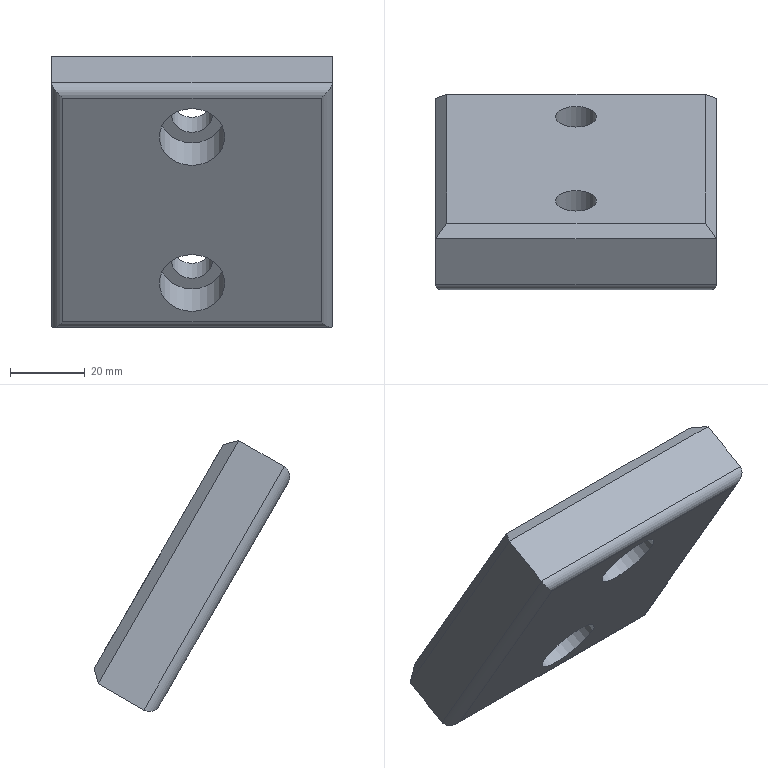Part | NX | features solid 2 | 1 solid | 20 faces | box 75 x 52.222 x 72.354 mm | volume 103324 mm3 | plane 12 | cylinder 8 | commonest cylinder face diameters 6 x4 11 x2 17.5 x2
STEP:
#1=CARTESIAN_POINT('',(-407.5,-502.515,-23.51));
#2=VERTEX_POINT('',#1);
#3=CARTESIAN_POINT('',(-407.5,-514.639,-30.51));
#4=VERTEX_POINT('',#3);
#5=CARTESIAN_POINT('',(-407.5,-499.917,-22.01));
#6=DIRECTION('',(0.,-0.866,-0.5));
#7=VECTOR('',#6,1000.);
#8=LINE('',#5,#7);
#9=EDGE_CURVE('',#2,#4,#8,.T.);
#10=ORIENTED_EDGE('',*,*,#9,.F.);
#11=CARTESIAN_POINT('',(-332.5,-502.515,-23.51));
#12=VERTEX_POINT('',#11);
#13=CARTESIAN_POINT('',(-332.5,-502.515,-23.51));
#14=DIRECTION('',(1.,0.,0.));
#15=VECTOR('',#14,1000.);
#16=LINE('',#13,#15);
#17=EDGE_CURVE('',#2,#12,#16,.T.);
#18=ORIENTED_EDGE('',*,*,#17,.T.);
#19=CARTESIAN_POINT('',(-332.5,-514.639,-30.51));
#20=VERTEX_POINT('',#19);
#21=CARTESIAN_POINT('',(-332.5,-499.917,-22.01));
#22=DIRECTION('',(0.,-0.866,-0.5));
#23=VECTOR('',#22,1000.);
#24=LINE('',#21,#23);
#25=EDGE_CURVE('',#12,#20,#24,.T.);
#26=ORIENTED_EDGE('',*,*,#25,.T.);
#27=CARTESIAN_POINT('',(-407.5,-514.639,-30.51));
#28=DIRECTION('',(-1.,0.,0.));
#29=VECTOR('',#28,1000.);
#30=LINE('',#27,#29);
#31=EDGE_CURVE('',#20,#4,#30,.T.);
#32=ORIENTED_EDGE('',*,*,#31,.T.);
#33=EDGE_LOOP('',(#10,#18,#26,#32));
#34=FACE_BOUND('',#33,.T.);
#35=CARTESIAN_POINT('',(-332.5,-499.917,-22.01));
#36=DIRECTION('',(0.,-0.5,0.866));
#37=DIRECTION('',(1.,0.,0.));
#38=AXIS2_PLACEMENT_3D('',#35,#36,#37);
#39=PLANE('',#38);
#40=ADVANCED_FACE('',(#34),#39,.F.);
#41=CARTESIAN_POINT('',(-407.5,-540.015,41.442));
#42=VERTEX_POINT('',#41);
#43=CARTESIAN_POINT('',(-407.5,-552.139,34.442));
#44=VERTEX_POINT('',#43);
#45=CARTESIAN_POINT('',(-407.5,-537.417,42.942));
#46=DIRECTION('',(0.,-0.866,-0.5));
#47=VECTOR('',#46,1000.);
#48=LINE('',#45,#47);
#49=EDGE_CURVE('',#42,#44,#48,.T.);
#50=ORIENTED_EDGE('',*,*,#49,.F.);
#51=CARTESIAN_POINT('',(-407.5,-502.515,-23.51));
#52=DIRECTION('',(0.,0.5,-0.866));
#53=VECTOR('',#52,1000.);
#54=LINE('',#51,#53);
#55=EDGE_CURVE('',#42,#2,#54,.T.);
#56=ORIENTED_EDGE('',*,*,#55,.T.);
#57=ORIENTED_EDGE('',*,*,#9,.T.);
#58=CARTESIAN_POINT('',(-407.5,-552.139,34.442));
#59=DIRECTION('',(0.,-0.5,0.866));
#60=VECTOR('',#59,1000.);
#61=LINE('',#58,#60);
#62=EDGE_CURVE('',#4,#44,#61,.T.);
#63=ORIENTED_EDGE('',*,*,#62,.T.);
#64=EDGE_LOOP('',(#50,#56,#57,#63));
#65=FACE_BOUND('',#64,.T.);
#66=CARTESIAN_POINT('',(-407.5,-499.917,-22.01));
#67=DIRECTION('',(1.,0.,0.));
#68=DIRECTION('',(0.,0.866,0.5));
#69=AXIS2_PLACEMENT_3D('',#66,#67,#68);
#70=PLANE('',#69);
#71=ADVANCED_FACE('',(#65),#70,.F.);
#72=CARTESIAN_POINT('',(-332.5,-540.015,41.442));
#73=VERTEX_POINT('',#72);
#74=CARTESIAN_POINT('',(-332.5,-552.139,34.442));
#75=VERTEX_POINT('',#74);
#76=CARTESIAN_POINT('',(-332.5,-537.417,42.942));
#77=DIRECTION('',(0.,-0.866,-0.5));
#78=VECTOR('',#77,1000.);
#79=LINE('',#76,#78);
#80=EDGE_CURVE('',#73,#75,#79,.T.);
#81=ORIENTED_EDGE('',*,*,#80,.F.);
#82=CARTESIAN_POINT('',(-407.5,-540.015,41.442));
#83=DIRECTION('',(-1.,0.,0.));
#84=VECTOR('',#83,1000.);
#85=LINE('',#82,#84);
#86=EDGE_CURVE('',#73,#42,#85,.T.);
#87=ORIENTED_EDGE('',*,*,#86,.T.);
#88=ORIENTED_EDGE('',*,*,#49,.T.);
#89=CARTESIAN_POINT('',(-332.5,-552.139,34.442));
#90=DIRECTION('',(1.,0.,0.));
#91=VECTOR('',#90,1000.);
#92=LINE('',#89,#91);
#93=EDGE_CURVE('',#44,#75,#92,.T.);
#94=ORIENTED_EDGE('',*,*,#93,.T.);
#95=EDGE_LOOP('',(#81,#87,#88,#94));
#96=FACE_BOUND('',#95,.T.);
#97=CARTESIAN_POINT('',(-407.5,-537.417,42.942));
#98=DIRECTION('',(0.,0.5,-0.866));
#99=DIRECTION('',(0.,0.866,0.5));
#100=AXIS2_PLACEMENT_3D('',#97,#98,#99);
#101=PLANE('',#100);
#102=ADVANCED_FACE('',(#96),#101,.F.);
#103=ORIENTED_EDGE('',*,*,#25,.F.);
#104=CARTESIAN_POINT('',(-332.5,-540.015,41.442));
#105=DIRECTION('',(0.,-0.5,0.866));
#106=VECTOR('',#105,1000.);
#107=LINE('',#104,#106);
#108=EDGE_CURVE('',#12,#73,#107,.T.);
#109=ORIENTED_EDGE('',*,*,#108,.T.);
#110=ORIENTED_EDGE('',*,*,#80,.T.);
#111=CARTESIAN_POINT('',(-332.5,-514.639,-30.51));
#112=DIRECTION('',(0.,0.5,-0.866));
#113=VECTOR('',#112,1000.);
#114=LINE('',#111,#113);
#115=EDGE_CURVE('',#75,#20,#114,.T.);
#116=ORIENTED_EDGE('',*,*,#115,.T.);
#117=EDGE_LOOP('',(#103,#109,#110,#116));
#118=FACE_BOUND('',#117,.T.);
#119=CARTESIAN_POINT('',(-332.5,-537.417,42.942));
#120=DIRECTION('',(-1.,0.,0.));
#121=DIRECTION('',(0.,-0.5,0.866));
#122=AXIS2_PLACEMENT_3D('',#119,#120,#121);
#123=PLANE('',#122);
#124=ADVANCED_FACE('',(#118),#123,.F.);
#125=CARTESIAN_POINT('',(-404.5,-501.417,-19.412));
#126=VERTEX_POINT('',#125);
#127=CARTESIAN_POINT('',(-404.5,-535.917,40.344));
#128=VERTEX_POINT('',#127);
#129=CARTESIAN_POINT('',(-404.5,-499.917,-22.01));
#130=DIRECTION('',(0.,-0.5,0.866));
#131=VECTOR('',#130,1000.);
#132=LINE('',#129,#131);
#133=EDGE_CURVE('',#126,#128,#132,.T.);
#134=ORIENTED_EDGE('',*,*,#133,.T.);
#135=CARTESIAN_POINT('',(-335.5,-535.917,40.344));
#136=VERTEX_POINT('',#135);
#137=CARTESIAN_POINT('',(-332.5,-535.917,40.344));
#138=DIRECTION('',(1.,0.,0.));
#139=VECTOR('',#138,1000.);
#140=LINE('',#137,#139);
#141=EDGE_CURVE('',#128,#136,#140,.T.);
#142=ORIENTED_EDGE('',*,*,#141,.T.);
#143=CARTESIAN_POINT('',(-335.5,-501.417,-19.412));
#144=VERTEX_POINT('',#143);
#145=CARTESIAN_POINT('',(-335.5,-499.917,-22.01));
#146=DIRECTION('',(0.,0.5,-0.866));
#147=VECTOR('',#146,1000.);
#148=LINE('',#145,#147);
#149=EDGE_CURVE('',#136,#144,#148,.T.);
#150=ORIENTED_EDGE('',*,*,#149,.T.);
#151=CARTESIAN_POINT('',(-332.5,-501.417,-19.412));
#152=DIRECTION('',(-1.,0.,0.));
#153=VECTOR('',#152,1000.);
#154=LINE('',#151,#153);
#155=EDGE_CURVE('',#144,#126,#154,.T.);
#156=ORIENTED_EDGE('',*,*,#155,.T.);
#157=EDGE_LOOP('',(#134,#142,#150,#156));
#158=FACE_BOUND('',#157,.T.);
#159=CARTESIAN_POINT('',(-370.,-527.167,25.189));
#160=VERTEX_POINT('',#159);
#161=CARTESIAN_POINT('',(-370.,-529.917,29.952));
#162=DIRECTION('',(0.,-0.866,-0.5));
#163=DIRECTION('',(0.,0.5,-0.866));
#164=AXIS2_PLACEMENT_3D('',#161,#162,#163);
#165=CIRCLE('',#164,5.5);
#166=EDGE_CURVE('',#160,#160,#165,.T.);
#167=ORIENTED_EDGE('',*,*,#166,.T.);
#168=EDGE_LOOP('',(#167));
#169=FACE_BOUND('',#168,.T.);
#170=CARTESIAN_POINT('',(-370.,-504.667,-13.782));
#171=VERTEX_POINT('',#170);
#172=CARTESIAN_POINT('',(-370.,-507.417,-9.019));
#173=DIRECTION('',(0.,-0.866,-0.5));
#174=DIRECTION('',(0.,0.5,-0.866));
#175=AXIS2_PLACEMENT_3D('',#172,#173,#174);
#176=CIRCLE('',#175,5.5);
#177=EDGE_CURVE('',#171,#171,#176,.T.);
#178=ORIENTED_EDGE('',*,*,#177,.T.);
#179=EDGE_LOOP('',(#178));
#180=FACE_BOUND('',#179,.T.);
#181=CARTESIAN_POINT('',(-332.5,-499.917,-22.01));
#182=DIRECTION('',(0.,-0.866,-0.5));
#183=DIRECTION('',(0.,0.5,-0.866));
#184=AXIS2_PLACEMENT_3D('',#181,#182,#183);
#185=PLANE('',#184);
#186=ADVANCED_FACE('',(#158,#169,#180),#185,.F.);
#187=CARTESIAN_POINT('',(-404.5,-518.737,-29.412));
#188=VERTEX_POINT('',#187);
#189=CARTESIAN_POINT('',(-335.5,-518.737,-29.412));
#190=VERTEX_POINT('',#189);
#191=CARTESIAN_POINT('',(-332.5,-518.737,-29.412));
#192=DIRECTION('',(-1.,0.,0.));
#193=VECTOR('',#192,1000.);
#194=LINE('',#191,#193);
#195=EDGE_CURVE('',#188,#190,#194,.F.);
#196=ORIENTED_EDGE('',*,*,#195,.T.);
#197=CARTESIAN_POINT('',(-335.5,-553.237,30.344));
#198=VERTEX_POINT('',#197);
#199=CARTESIAN_POINT('',(-335.5,-554.737,32.942));
#200=DIRECTION('',(0.,0.5,-0.866));
#201=VECTOR('',#200,1000.);
#202=LINE('',#199,#201);
#203=EDGE_CURVE('',#190,#198,#202,.F.);
#204=ORIENTED_EDGE('',*,*,#203,.T.);
#205=CARTESIAN_POINT('',(-404.5,-553.237,30.344));
#206=VERTEX_POINT('',#205);
#207=CARTESIAN_POINT('',(-407.5,-553.237,30.344));
#208=DIRECTION('',(1.,0.,0.));
#209=VECTOR('',#208,1000.);
#210=LINE('',#207,#209);
#211=EDGE_CURVE('',#198,#206,#210,.F.);
#212=ORIENTED_EDGE('',*,*,#211,.T.);
#213=CARTESIAN_POINT('',(-404.5,-517.237,-32.01));
#214=DIRECTION('',(0.,-0.5,0.866));
#215=VECTOR('',#214,1000.);
#216=LINE('',#213,#215);
#217=EDGE_CURVE('',#206,#188,#216,.F.);
#218=ORIENTED_EDGE('',*,*,#217,.T.);
#219=EDGE_LOOP('',(#196,#204,#212,#218));
#220=FACE_BOUND('',#219,.T.);
#221=CARTESIAN_POINT('',(-370.,-551.612,27.53));
#222=VERTEX_POINT('',#221);
#223=CARTESIAN_POINT('',(-370.,-547.237,19.952));
#224=DIRECTION('',(0.,0.866,0.5));
#225=DIRECTION('',(0.,-0.5,0.866));
#226=AXIS2_PLACEMENT_3D('',#223,#224,#225);
#227=CIRCLE('',#226,8.75);
#228=EDGE_CURVE('',#222,#222,#227,.T.);
#229=ORIENTED_EDGE('',*,*,#228,.T.);
#230=EDGE_LOOP('',(#229));
#231=FACE_BOUND('',#230,.T.);
#232=CARTESIAN_POINT('',(-370.,-529.112,-11.442));
#233=VERTEX_POINT('',#232);
#234=CARTESIAN_POINT('',(-370.,-524.737,-19.019));
#235=DIRECTION('',(0.,0.866,0.5));
#236=DIRECTION('',(0.,-0.5,0.866));
#237=AXIS2_PLACEMENT_3D('',#234,#235,#236);
#238=CIRCLE('',#237,8.75);
#239=EDGE_CURVE('',#233,#233,#238,.T.);
#240=ORIENTED_EDGE('',*,*,#239,.T.);
#241=EDGE_LOOP('',(#240));
#242=FACE_BOUND('',#241,.T.);
#243=CARTESIAN_POINT('',(-332.5,-517.237,-32.01));
#244=DIRECTION('',(0.,-0.866,-0.5));
#245=DIRECTION('',(0.,0.5,-0.866));
#246=AXIS2_PLACEMENT_3D('',#243,#244,#245);
#247=PLANE('',#246);
#248=ADVANCED_FACE('',(#220,#231,#242),#247,.T.);
#249=CARTESIAN_POINT('',(-370.,-517.095,-8.256));
#250=VERTEX_POINT('',#249);
#251=CARTESIAN_POINT('',(-370.,-514.345,-13.019));
#252=DIRECTION('',(0.,0.866,0.5));
#253=DIRECTION('',(0.,-0.5,0.866));
#254=AXIS2_PLACEMENT_3D('',#251,#252,#253);
#255=CIRCLE('',#254,5.5);
#256=EDGE_CURVE('',#250,#250,#255,.T.);
#257=ORIENTED_EDGE('',*,*,#256,.F.);
#258=EDGE_LOOP('',(#257));
#259=FACE_BOUND('',#258,.T.);
#260=ORIENTED_EDGE('',*,*,#177,.F.);
#261=EDGE_LOOP('',(#260));
#262=FACE_BOUND('',#261,.T.);
#263=CARTESIAN_POINT('',(-370.,-481.436,5.981));
#264=DIRECTION('',(0.,0.866,0.5));
#265=DIRECTION('',(0.,-0.5,0.866));
#266=AXIS2_PLACEMENT_3D('',#263,#264,#265);
#267=CYLINDRICAL_SURFACE('',#266,5.5);
#268=ADVANCED_FACE('',(#259,#262),#267,.F.);
#269=ORIENTED_EDGE('',*,*,#256,.T.);
#270=EDGE_LOOP('',(#269));
#271=FACE_BOUND('',#270,.T.);
#272=CARTESIAN_POINT('',(-370.,-518.72,-5.442));
#273=VERTEX_POINT('',#272);
#274=CARTESIAN_POINT('',(-370.,-514.345,-13.019));
#275=DIRECTION('',(0.,0.866,0.5));
#276=DIRECTION('',(0.,-0.5,0.866));
#277=AXIS2_PLACEMENT_3D('',#274,#275,#276);
#278=CIRCLE('',#277,8.75);
#279=EDGE_CURVE('',#273,#273,#278,.T.);
#280=ORIENTED_EDGE('',*,*,#279,.F.);
#281=EDGE_LOOP('',(#280));
#282=FACE_BOUND('',#281,.T.);
#283=CARTESIAN_POINT('',(-370.,-514.345,-13.019));
#284=DIRECTION('',(0.,0.866,0.5));
#285=DIRECTION('',(0.,-0.5,0.866));
#286=AXIS2_PLACEMENT_3D('',#283,#284,#285);
#287=PLANE('',#286);
#288=ADVANCED_FACE('',(#271,#282),#287,.F.);
#289=ORIENTED_EDGE('',*,*,#279,.T.);
#290=EDGE_LOOP('',(#289));
#291=FACE_BOUND('',#290,.T.);
#292=ORIENTED_EDGE('',*,*,#239,.F.);
#293=EDGE_LOOP('',(#292));
#294=FACE_BOUND('',#293,.T.);
#295=CARTESIAN_POINT('',(-370.,-524.737,-19.019));
#296=DIRECTION('',(0.,0.866,0.5));
#297=DIRECTION('',(0.,-0.5,0.866));
#298=AXIS2_PLACEMENT_3D('',#295,#296,#297);
#299=CYLINDRICAL_SURFACE('',#298,8.75);
#300=ADVANCED_FACE('',(#291,#294),#299,.F.);
#301=CARTESIAN_POINT('',(-370.,-539.595,30.715));
#302=VERTEX_POINT('',#301);
#303=CARTESIAN_POINT('',(-370.,-536.845,25.952));
#304=DIRECTION('',(0.,0.866,0.5));
#305=DIRECTION('',(0.,-0.5,0.866));
#306=AXIS2_PLACEMENT_3D('',#303,#304,#305);
#307=CIRCLE('',#306,5.5);
#308=EDGE_CURVE('',#302,#302,#307,.T.);
#309=ORIENTED_EDGE('',*,*,#308,.F.);
#310=EDGE_LOOP('',(#309));
#311=FACE_BOUND('',#310,.T.);
#312=ORIENTED_EDGE('',*,*,#166,.F.);
#313=EDGE_LOOP('',(#312));
#314=FACE_BOUND('',#313,.T.);
#315=CARTESIAN_POINT('',(-370.,-503.936,44.952));
#316=DIRECTION('',(0.,0.866,0.5));
#317=DIRECTION('',(0.,-0.5,0.866));
#318=AXIS2_PLACEMENT_3D('',#315,#316,#317);
#319=CYLINDRICAL_SURFACE('',#318,5.5);
#320=ADVANCED_FACE('',(#311,#314),#319,.F.);
#321=ORIENTED_EDGE('',*,*,#308,.T.);
#322=EDGE_LOOP('',(#321));
#323=FACE_BOUND('',#322,.T.);
#324=CARTESIAN_POINT('',(-370.,-541.22,33.53));
#325=VERTEX_POINT('',#324);
#326=CARTESIAN_POINT('',(-370.,-536.845,25.952));
#327=DIRECTION('',(0.,0.866,0.5));
#328=DIRECTION('',(0.,-0.5,0.866));
#329=AXIS2_PLACEMENT_3D('',#326,#327,#328);
#330=CIRCLE('',#329,8.75);
#331=EDGE_CURVE('',#325,#325,#330,.T.);
#332=ORIENTED_EDGE('',*,*,#331,.F.);
#333=EDGE_LOOP('',(#332));
#334=FACE_BOUND('',#333,.T.);
#335=CARTESIAN_POINT('',(-370.,-536.845,25.952));
#336=DIRECTION('',(0.,0.866,0.5));
#337=DIRECTION('',(0.,-0.5,0.866));
#338=AXIS2_PLACEMENT_3D('',#335,#336,#337);
#339=PLANE('',#338);
#340=ADVANCED_FACE('',(#323,#334),#339,.F.);
#341=ORIENTED_EDGE('',*,*,#331,.T.);
#342=EDGE_LOOP('',(#341));
#343=FACE_BOUND('',#342,.T.);
#344=ORIENTED_EDGE('',*,*,#228,.F.);
#345=EDGE_LOOP('',(#344));
#346=FACE_BOUND('',#345,.T.);
#347=CARTESIAN_POINT('',(-370.,-547.237,19.952));
#348=DIRECTION('',(0.,0.866,0.5));
#349=DIRECTION('',(0.,-0.5,0.866));
#350=AXIS2_PLACEMENT_3D('',#347,#348,#349);
#351=CYLINDRICAL_SURFACE('',#350,8.75);
#352=ADVANCED_FACE('',(#343,#346),#351,.F.);
#353=CARTESIAN_POINT('',(-404.5,-516.139,-27.912));
#354=DIRECTION('',(0.7071,0.3536,-0.6124));
#355=DIRECTION('',(0.7071,-0.3536,0.6124));
#356=AXIS2_PLACEMENT_3D('',#353,#354,#355);
#357=ELLIPSE('',#356,4.243,3.);
#358=EDGE_CURVE('',#188,#4,#357,.T.);
#359=ORIENTED_EDGE('',*,*,#358,.F.);
#360=ORIENTED_EDGE('',*,*,#217,.F.);
#361=CARTESIAN_POINT('',(-404.5,-550.639,31.844));
#362=DIRECTION('',(-0.7071,0.3536,-0.6124));
#363=DIRECTION('',(0.7071,0.3536,-0.6124));
#364=AXIS2_PLACEMENT_3D('',#361,#362,#363);
#365=ELLIPSE('',#364,4.243,3.);
#366=EDGE_CURVE('',#44,#206,#365,.F.);
#367=ORIENTED_EDGE('',*,*,#366,.F.);
#368=ORIENTED_EDGE('',*,*,#62,.F.);
#369=EDGE_LOOP('',(#359,#360,#367,#368));
#370=FACE_BOUND('',#369,.T.);
#371=CARTESIAN_POINT('',(-404.5,-514.639,-30.51));
#372=DIRECTION('',(0.,0.5,-0.866));
#373=DIRECTION('',(0.,0.866,0.5));
#374=AXIS2_PLACEMENT_3D('',#371,#372,#373);
#375=CYLINDRICAL_SURFACE('',#374,3.);
#376=ADVANCED_FACE('',(#370),#375,.T.);
#377=ORIENTED_EDGE('',*,*,#366,.T.);
#378=ORIENTED_EDGE('',*,*,#211,.F.);
#379=CARTESIAN_POINT('',(-335.5,-550.639,31.844));
#380=DIRECTION('',(-0.7071,-0.3536,0.6124));
#381=DIRECTION('',(-0.7071,0.3536,-0.6124));
#382=AXIS2_PLACEMENT_3D('',#379,#380,#381);
#383=ELLIPSE('',#382,4.243,3.);
#384=EDGE_CURVE('',#75,#198,#383,.F.);
#385=ORIENTED_EDGE('',*,*,#384,.F.);
#386=ORIENTED_EDGE('',*,*,#93,.F.);
#387=EDGE_LOOP('',(#377,#378,#385,#386));
#388=FACE_BOUND('',#387,.T.);
#389=CARTESIAN_POINT('',(-407.5,-550.639,31.844));
#390=DIRECTION('',(-1.,0.,0.));
#391=DIRECTION('',(0.,-0.866,-0.5));
#392=AXIS2_PLACEMENT_3D('',#389,#390,#391);
#393=CYLINDRICAL_SURFACE('',#392,3.);
#394=ADVANCED_FACE('',(#388),#393,.T.);
#395=ORIENTED_EDGE('',*,*,#358,.T.);
#396=ORIENTED_EDGE('',*,*,#31,.F.);
#397=CARTESIAN_POINT('',(-335.5,-516.139,-27.912));
#398=DIRECTION('',(0.7071,-0.3536,0.6124));
#399=DIRECTION('',(0.7071,0.3536,-0.6124));
#400=AXIS2_PLACEMENT_3D('',#397,#398,#399);
#401=ELLIPSE('',#400,4.243,3.);
#402=EDGE_CURVE('',#190,#20,#401,.T.);
#403=ORIENTED_EDGE('',*,*,#402,.F.);
#404=ORIENTED_EDGE('',*,*,#195,.F.);
#405=EDGE_LOOP('',(#395,#396,#403,#404));
#406=FACE_BOUND('',#405,.T.);
#407=CARTESIAN_POINT('',(-332.5,-516.139,-27.912));
#408=DIRECTION('',(1.,0.,0.));
#409=DIRECTION('',(0.,0.5,-0.866));
#410=AXIS2_PLACEMENT_3D('',#407,#408,#409);
#411=CYLINDRICAL_SURFACE('',#410,3.);
#412=ADVANCED_FACE('',(#406),#411,.T.);
#413=ORIENTED_EDGE('',*,*,#384,.T.);
#414=ORIENTED_EDGE('',*,*,#203,.F.);
#415=ORIENTED_EDGE('',*,*,#402,.T.);
#416=ORIENTED_EDGE('',*,*,#115,.F.);
#417=EDGE_LOOP('',(#413,#414,#415,#416));
#418=FACE_BOUND('',#417,.T.);
#419=CARTESIAN_POINT('',(-335.5,-552.139,34.442));
#420=DIRECTION('',(0.,-0.5,0.866));
#421=DIRECTION('',(1.,0.,0.));
#422=AXIS2_PLACEMENT_3D('',#419,#420,#421);
#423=CYLINDRICAL_SURFACE('',#422,3.);
#424=ADVANCED_FACE('',(#418),#423,.T.);
#425=CARTESIAN_POINT('',(-334.5,-501.783,-20.778));
#426=DIRECTION('',(-0.5774,0.2113,0.7887));
#427=VECTOR('',#426,1000.);
#428=LINE('',#425,#427);
#429=EDGE_CURVE('',#12,#144,#428,.T.);
#430=ORIENTED_EDGE('',*,*,#429,.F.);
#431=ORIENTED_EDGE('',*,*,#17,.F.);
#432=CARTESIAN_POINT('',(-380.5,-492.632,13.373));
#433=DIRECTION('',(0.5774,0.2113,0.7887));
#434=VECTOR('',#433,1000.);
#435=LINE('',#432,#434);
#436=EDGE_CURVE('',#126,#2,#435,.F.);
#437=ORIENTED_EDGE('',*,*,#436,.F.);
#438=ORIENTED_EDGE('',*,*,#155,.F.);
#439=EDGE_LOOP('',(#430,#431,#437,#438));
#440=FACE_BOUND('',#439,.T.);
#441=CARTESIAN_POINT('',(-332.5,-501.417,-19.412));
#442=DIRECTION('',(0.,-0.9659,0.2588));
#443=DIRECTION('',(0.,-0.2588,-0.9659));
#444=AXIS2_PLACEMENT_3D('',#441,#442,#443);
#445=PLANE('',#444);
#446=ADVANCED_FACE('',(#440),#445,.F.);
#447=ORIENTED_EDGE('',*,*,#436,.T.);
#448=ORIENTED_EDGE('',*,*,#55,.F.);
#449=CARTESIAN_POINT('',(-380.5,-503.132,31.56));
#450=DIRECTION('',(0.5774,0.7887,-0.2113));
#451=VECTOR('',#450,1000.);
#452=LINE('',#449,#451);
#453=EDGE_CURVE('',#128,#42,#452,.F.);
#454=ORIENTED_EDGE('',*,*,#453,.F.);
#455=ORIENTED_EDGE('',*,*,#133,.F.);
#456=EDGE_LOOP('',(#447,#448,#454,#455));
#457=FACE_BOUND('',#456,.T.);
#458=CARTESIAN_POINT('',(-404.5,-499.917,-22.01));
#459=DIRECTION('',(0.7071,-0.6124,-0.3536));
#460=DIRECTION('',(0.7071,0.6124,0.3536));
#461=AXIS2_PLACEMENT_3D('',#458,#459,#460);
#462=PLANE('',#461);
#463=ADVANCED_FACE('',(#457),#462,.F.);
#464=ORIENTED_EDGE('',*,*,#429,.T.);
#465=ORIENTED_EDGE('',*,*,#149,.F.);
#466=CARTESIAN_POINT('',(-359.5,-503.132,31.56));
#467=DIRECTION('',(0.5774,-0.7887,0.2113));
#468=VECTOR('',#467,1000.);
#469=LINE('',#466,#468);
#470=EDGE_CURVE('',#73,#136,#469,.F.);
#471=ORIENTED_EDGE('',*,*,#470,.F.);
#472=ORIENTED_EDGE('',*,*,#108,.F.);
#473=EDGE_LOOP('',(#464,#465,#471,#472));
#474=FACE_BOUND('',#473,.T.);
#475=CARTESIAN_POINT('',(-335.5,-499.917,-22.01));
#476=DIRECTION('',(-0.7071,-0.6124,-0.3536));
#477=DIRECTION('',(0.7071,-0.6124,-0.3536));
#478=AXIS2_PLACEMENT_3D('',#475,#476,#477);
#479=PLANE('',#478);
#480=ADVANCED_FACE('',(#474),#479,.F.);
#481=ORIENTED_EDGE('',*,*,#453,.T.);
#482=ORIENTED_EDGE('',*,*,#86,.F.);
#483=ORIENTED_EDGE('',*,*,#470,.T.);
#484=ORIENTED_EDGE('',*,*,#141,.F.);
#485=EDGE_LOOP('',(#481,#482,#483,#484));
#486=FACE_BOUND('',#485,.T.);
#487=CARTESIAN_POINT('',(-332.5,-535.917,40.344));
#488=DIRECTION('',(0.,-0.2588,-0.9659));
#489=DIRECTION('',(0.,0.9659,-0.2588));
#490=AXIS2_PLACEMENT_3D('',#487,#488,#489);
#491=PLANE('',#490);
#492=ADVANCED_FACE('',(#486),#491,.F.);
#493=CLOSED_SHELL('',(#40,#71,#102,#124,#186,#248,#268,#288,#300,#320,#340,#352,#376,#394,#412,#424,#446,#463,#480,#492));
#494=MANIFOLD_SOLID_BREP('',#493);
#495=(LENGTH_UNIT()NAMED_UNIT(*)SI_UNIT(.MILLI.,.METRE.));
#496=UNCERTAINTY_MEASURE_WITH_UNIT(LENGTH_MEASURE(0.00001),#495,'','');
#497=(NAMED_UNIT(*)PLANE_ANGLE_UNIT()SI_UNIT($,.RADIAN.));
#498=(NAMED_UNIT(*)SI_UNIT($,.STERADIAN.)SOLID_ANGLE_UNIT());
#499=(GEOMETRIC_REPRESENTATION_CONTEXT(3)GLOBAL_UNCERTAINTY_ASSIGNED_CONTEXT((#496))GLOBAL_UNIT_ASSIGNED_CONTEXT((#495,#497,#498))REPRESENTATION_CONTEXT('',''));
#500=ADVANCED_BREP_SHAPE_REPRESENTATION('',(#494),#499);